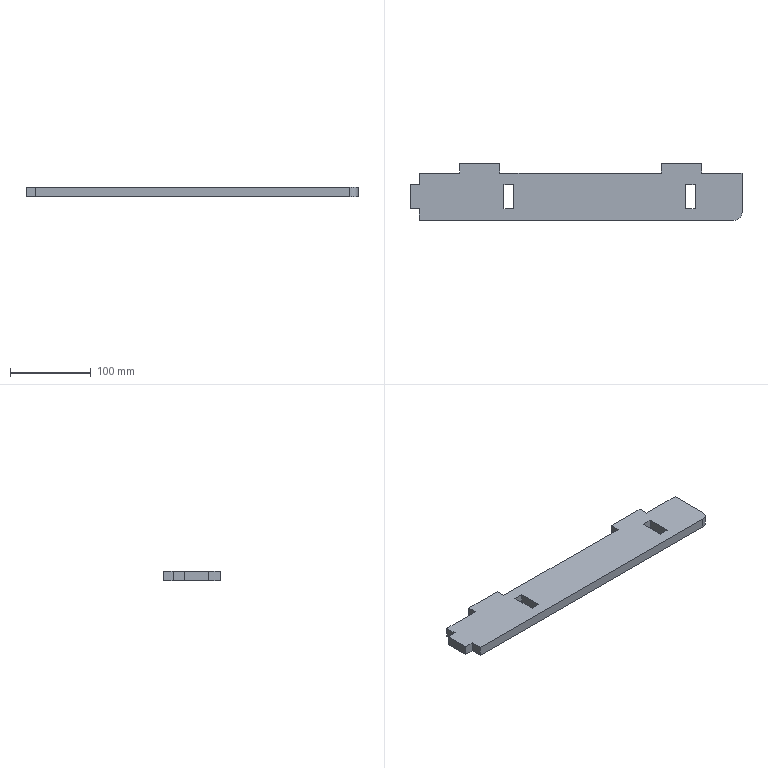Part | SolidWorks | features FlatPattern 1, SMBaseFlange 1, SheetMetal 1 | 1 solid | 27 faces | box 411.5 x 70 x 12 mm | volume 289842 mm3 | plane 26 | cylinder 1 | commonest cylinder face diameters 20 x1
STEP:
#1=CARTESIAN_POINT('',(166.972,-124.118,0.));
#2=VERTEX_POINT('',#1);
#3=CARTESIAN_POINT('',(166.972,-138.368,0.));
#4=VERTEX_POINT('',#3);
#5=CARTESIAN_POINT('',(166.972,-124.118,0.));
#6=DIRECTION('',(0.,-1.,0.));
#7=VECTOR('',#6,1000.);
#8=LINE('',#5,#7);
#9=EDGE_CURVE('',#2,#4,#8,.T.);
#10=ORIENTED_EDGE('',*,*,#9,.F.);
#11=CARTESIAN_POINT('',(166.972,-124.118,-12.));
#12=VERTEX_POINT('',#11);
#13=CARTESIAN_POINT('',(166.972,-124.118,-12.));
#14=DIRECTION('',(0.,0.,1.));
#15=VECTOR('',#14,1000.);
#16=LINE('',#13,#15);
#17=EDGE_CURVE('',#12,#2,#16,.T.);
#18=ORIENTED_EDGE('',*,*,#17,.F.);
#19=CARTESIAN_POINT('',(166.972,-138.368,-12.));
#20=VERTEX_POINT('',#19);
#21=CARTESIAN_POINT('',(166.972,-124.118,-12.));
#22=DIRECTION('',(0.,-1.,0.));
#23=VECTOR('',#22,1000.);
#24=LINE('',#21,#23);
#25=EDGE_CURVE('',#12,#20,#24,.T.);
#26=ORIENTED_EDGE('',*,*,#25,.T.);
#27=CARTESIAN_POINT('',(166.972,-138.368,-12.));
#28=DIRECTION('',(0.,0.,1.));
#29=VECTOR('',#28,1000.);
#30=LINE('',#27,#29);
#31=EDGE_CURVE('',#20,#4,#30,.T.);
#32=ORIENTED_EDGE('',*,*,#31,.T.);
#33=EDGE_LOOP('',(#10,#18,#26,#32));
#34=FACE_OUTER_BOUND('',#33,.T.);
#35=CARTESIAN_POINT('',(166.972,-124.118,-12.));
#36=DIRECTION('',(-1.,0.,0.));
#37=DIRECTION('',(0.,0.,1.));
#38=AXIS2_PLACEMENT_3D('',#35,#36,#37);
#39=PLANE('',#38);
#40=ADVANCED_FACE('',(#34),#39,.T.);
#41=CARTESIAN_POINT('',(216.972,-124.118,0.));
#42=VERTEX_POINT('',#41);
#43=CARTESIAN_POINT('',(166.972,-124.118,0.));
#44=DIRECTION('',(-1.,0.,0.));
#45=VECTOR('',#44,1000.);
#46=LINE('',#43,#45);
#47=EDGE_CURVE('',#42,#2,#46,.T.);
#48=ORIENTED_EDGE('',*,*,#47,.F.);
#49=CARTESIAN_POINT('',(216.972,-124.118,-12.));
#50=VERTEX_POINT('',#49);
#51=CARTESIAN_POINT('',(216.972,-124.118,-12.));
#52=DIRECTION('',(0.,0.,1.));
#53=VECTOR('',#52,1000.);
#54=LINE('',#51,#53);
#55=EDGE_CURVE('',#50,#42,#54,.T.);
#56=ORIENTED_EDGE('',*,*,#55,.F.);
#57=CARTESIAN_POINT('',(166.972,-124.118,-12.));
#58=DIRECTION('',(-1.,0.,0.));
#59=VECTOR('',#58,1000.);
#60=LINE('',#57,#59);
#61=EDGE_CURVE('',#50,#12,#60,.T.);
#62=ORIENTED_EDGE('',*,*,#61,.T.);
#63=ORIENTED_EDGE('',*,*,#17,.T.);
#64=EDGE_LOOP('',(#48,#56,#62,#63));
#65=FACE_OUTER_BOUND('',#64,.T.);
#66=CARTESIAN_POINT('',(166.972,-124.118,-12.));
#67=DIRECTION('',(0.,1.,0.));
#68=DIRECTION('',(-1.,0.,0.));
#69=AXIS2_PLACEMENT_3D('',#66,#67,#68);
#70=PLANE('',#69);
#71=ADVANCED_FACE('',(#65),#70,.T.);
#72=CARTESIAN_POINT('',(216.972,-112.618,0.));
#73=VERTEX_POINT('',#72);
#74=CARTESIAN_POINT('',(216.972,-112.618,0.));
#75=DIRECTION('',(0.,-1.,0.));
#76=VECTOR('',#75,1000.);
#77=LINE('',#74,#76);
#78=EDGE_CURVE('',#73,#42,#77,.T.);
#79=ORIENTED_EDGE('',*,*,#78,.F.);
#80=CARTESIAN_POINT('',(216.972,-112.618,-12.));
#81=VERTEX_POINT('',#80);
#82=CARTESIAN_POINT('',(216.972,-112.618,-12.));
#83=DIRECTION('',(0.,0.,1.));
#84=VECTOR('',#83,1000.);
#85=LINE('',#82,#84);
#86=EDGE_CURVE('',#81,#73,#85,.T.);
#87=ORIENTED_EDGE('',*,*,#86,.F.);
#88=CARTESIAN_POINT('',(216.972,-112.618,-12.));
#89=DIRECTION('',(0.,-1.,0.));
#90=VECTOR('',#89,1000.);
#91=LINE('',#88,#90);
#92=EDGE_CURVE('',#81,#50,#91,.T.);
#93=ORIENTED_EDGE('',*,*,#92,.T.);
#94=ORIENTED_EDGE('',*,*,#55,.T.);
#95=EDGE_LOOP('',(#79,#87,#93,#94));
#96=FACE_OUTER_BOUND('',#95,.T.);
#97=CARTESIAN_POINT('',(216.972,-112.618,-12.));
#98=DIRECTION('',(-1.,0.,0.));
#99=DIRECTION('',(0.,0.,1.));
#100=AXIS2_PLACEMENT_3D('',#97,#98,#99);
#101=PLANE('',#100);
#102=ADVANCED_FACE('',(#96),#101,.T.);
#103=CARTESIAN_POINT('',(266.972,-112.618,0.));
#104=VERTEX_POINT('',#103);
#105=CARTESIAN_POINT('',(266.972,-112.618,0.));
#106=DIRECTION('',(-1.,0.,0.));
#107=VECTOR('',#106,1000.);
#108=LINE('',#105,#107);
#109=EDGE_CURVE('',#104,#73,#108,.T.);
#110=ORIENTED_EDGE('',*,*,#109,.F.);
#111=CARTESIAN_POINT('',(266.972,-112.618,-12.));
#112=VERTEX_POINT('',#111);
#113=CARTESIAN_POINT('',(266.972,-112.618,-12.));
#114=DIRECTION('',(0.,0.,1.));
#115=VECTOR('',#114,1000.);
#116=LINE('',#113,#115);
#117=EDGE_CURVE('',#112,#104,#116,.T.);
#118=ORIENTED_EDGE('',*,*,#117,.F.);
#119=CARTESIAN_POINT('',(266.972,-112.618,-12.));
#120=DIRECTION('',(-1.,0.,0.));
#121=VECTOR('',#120,1000.);
#122=LINE('',#119,#121);
#123=EDGE_CURVE('',#112,#81,#122,.T.);
#124=ORIENTED_EDGE('',*,*,#123,.T.);
#125=ORIENTED_EDGE('',*,*,#86,.T.);
#126=EDGE_LOOP('',(#110,#118,#124,#125));
#127=FACE_OUTER_BOUND('',#126,.T.);
#128=CARTESIAN_POINT('',(266.972,-112.618,-12.));
#129=DIRECTION('',(0.,1.,0.));
#130=DIRECTION('',(0.,0.,1.));
#131=AXIS2_PLACEMENT_3D('',#128,#129,#130);
#132=PLANE('',#131);
#133=ADVANCED_FACE('',(#127),#132,.T.);
#134=CARTESIAN_POINT('',(266.972,-124.118,0.));
#135=VERTEX_POINT('',#134);
#136=CARTESIAN_POINT('',(266.972,-124.118,0.));
#137=DIRECTION('',(0.,1.,0.));
#138=VECTOR('',#137,1000.);
#139=LINE('',#136,#138);
#140=EDGE_CURVE('',#135,#104,#139,.T.);
#141=ORIENTED_EDGE('',*,*,#140,.F.);
#142=CARTESIAN_POINT('',(266.972,-124.118,-12.));
#143=VERTEX_POINT('',#142);
#144=CARTESIAN_POINT('',(266.972,-124.118,-12.));
#145=DIRECTION('',(0.,0.,1.));
#146=VECTOR('',#145,1000.);
#147=LINE('',#144,#146);
#148=EDGE_CURVE('',#143,#135,#147,.T.);
#149=ORIENTED_EDGE('',*,*,#148,.F.);
#150=CARTESIAN_POINT('',(266.972,-124.118,-12.));
#151=DIRECTION('',(0.,1.,0.));
#152=VECTOR('',#151,1000.);
#153=LINE('',#150,#152);
#154=EDGE_CURVE('',#143,#112,#153,.T.);
#155=ORIENTED_EDGE('',*,*,#154,.T.);
#156=ORIENTED_EDGE('',*,*,#117,.T.);
#157=EDGE_LOOP('',(#141,#149,#155,#156));
#158=FACE_OUTER_BOUND('',#157,.T.);
#159=CARTESIAN_POINT('',(266.972,-124.118,-12.));
#160=DIRECTION('',(1.,0.,0.));
#161=DIRECTION('',(0.,1.,0.));
#162=AXIS2_PLACEMENT_3D('',#159,#160,#161);
#163=PLANE('',#162);
#164=ADVANCED_FACE('',(#158),#163,.T.);
#165=CARTESIAN_POINT('',(466.972,-124.118,0.));
#166=VERTEX_POINT('',#165);
#167=CARTESIAN_POINT('',(266.972,-124.118,0.));
#168=DIRECTION('',(-1.,0.,0.));
#169=VECTOR('',#168,1000.);
#170=LINE('',#167,#169);
#171=EDGE_CURVE('',#166,#135,#170,.T.);
#172=ORIENTED_EDGE('',*,*,#171,.F.);
#173=CARTESIAN_POINT('',(466.972,-124.118,-12.));
#174=VERTEX_POINT('',#173);
#175=CARTESIAN_POINT('',(466.972,-124.118,-12.));
#176=DIRECTION('',(0.,0.,1.));
#177=VECTOR('',#176,1000.);
#178=LINE('',#175,#177);
#179=EDGE_CURVE('',#174,#166,#178,.T.);
#180=ORIENTED_EDGE('',*,*,#179,.F.);
#181=CARTESIAN_POINT('',(266.972,-124.118,-12.));
#182=DIRECTION('',(-1.,0.,0.));
#183=VECTOR('',#182,1000.);
#184=LINE('',#181,#183);
#185=EDGE_CURVE('',#174,#143,#184,.T.);
#186=ORIENTED_EDGE('',*,*,#185,.T.);
#187=ORIENTED_EDGE('',*,*,#148,.T.);
#188=EDGE_LOOP('',(#172,#180,#186,#187));
#189=FACE_OUTER_BOUND('',#188,.T.);
#190=CARTESIAN_POINT('',(266.972,-124.118,-12.));
#191=DIRECTION('',(0.,1.,0.));
#192=DIRECTION('',(0.,0.,1.));
#193=AXIS2_PLACEMENT_3D('',#190,#191,#192);
#194=PLANE('',#193);
#195=ADVANCED_FACE('',(#189),#194,.T.);
#196=CARTESIAN_POINT('',(466.972,-112.618,0.));
#197=VERTEX_POINT('',#196);
#198=CARTESIAN_POINT('',(466.972,-112.618,0.));
#199=DIRECTION('',(0.,-1.,0.));
#200=VECTOR('',#199,1000.);
#201=LINE('',#198,#200);
#202=EDGE_CURVE('',#197,#166,#201,.T.);
#203=ORIENTED_EDGE('',*,*,#202,.F.);
#204=CARTESIAN_POINT('',(466.972,-112.618,-12.));
#205=VERTEX_POINT('',#204);
#206=CARTESIAN_POINT('',(466.972,-112.618,-12.));
#207=DIRECTION('',(0.,0.,1.));
#208=VECTOR('',#207,1000.);
#209=LINE('',#206,#208);
#210=EDGE_CURVE('',#205,#197,#209,.T.);
#211=ORIENTED_EDGE('',*,*,#210,.F.);
#212=CARTESIAN_POINT('',(466.972,-112.618,-12.));
#213=DIRECTION('',(0.,-1.,0.));
#214=VECTOR('',#213,1000.);
#215=LINE('',#212,#214);
#216=EDGE_CURVE('',#205,#174,#215,.T.);
#217=ORIENTED_EDGE('',*,*,#216,.T.);
#218=ORIENTED_EDGE('',*,*,#179,.T.);
#219=EDGE_LOOP('',(#203,#211,#217,#218));
#220=FACE_OUTER_BOUND('',#219,.T.);
#221=CARTESIAN_POINT('',(466.972,-112.618,-12.));
#222=DIRECTION('',(-1.,0.,0.));
#223=DIRECTION('',(0.,0.,1.));
#224=AXIS2_PLACEMENT_3D('',#221,#222,#223);
#225=PLANE('',#224);
#226=ADVANCED_FACE('',(#220),#225,.T.);
#227=CARTESIAN_POINT('',(516.972,-112.618,0.));
#228=VERTEX_POINT('',#227);
#229=CARTESIAN_POINT('',(516.972,-112.618,0.));
#230=DIRECTION('',(-1.,0.,0.));
#231=VECTOR('',#230,1000.);
#232=LINE('',#229,#231);
#233=EDGE_CURVE('',#228,#197,#232,.T.);
#234=ORIENTED_EDGE('',*,*,#233,.F.);
#235=CARTESIAN_POINT('',(516.972,-112.618,-12.));
#236=VERTEX_POINT('',#235);
#237=CARTESIAN_POINT('',(516.972,-112.618,-12.));
#238=DIRECTION('',(0.,0.,1.));
#239=VECTOR('',#238,1000.);
#240=LINE('',#237,#239);
#241=EDGE_CURVE('',#236,#228,#240,.T.);
#242=ORIENTED_EDGE('',*,*,#241,.F.);
#243=CARTESIAN_POINT('',(516.972,-112.618,-12.));
#244=DIRECTION('',(-1.,0.,0.));
#245=VECTOR('',#244,1000.);
#246=LINE('',#243,#245);
#247=EDGE_CURVE('',#236,#205,#246,.T.);
#248=ORIENTED_EDGE('',*,*,#247,.T.);
#249=ORIENTED_EDGE('',*,*,#210,.T.);
#250=EDGE_LOOP('',(#234,#242,#248,#249));
#251=FACE_OUTER_BOUND('',#250,.T.);
#252=CARTESIAN_POINT('',(516.972,-112.618,-12.));
#253=DIRECTION('',(0.,1.,0.));
#254=DIRECTION('',(-1.,0.,0.));
#255=AXIS2_PLACEMENT_3D('',#252,#253,#254);
#256=PLANE('',#255);
#257=ADVANCED_FACE('',(#251),#256,.T.);
#258=CARTESIAN_POINT('',(516.972,-124.118,0.));
#259=VERTEX_POINT('',#258);
#260=CARTESIAN_POINT('',(516.972,-124.118,0.));
#261=DIRECTION('',(0.,1.,0.));
#262=VECTOR('',#261,1000.);
#263=LINE('',#260,#262);
#264=EDGE_CURVE('',#259,#228,#263,.T.);
#265=ORIENTED_EDGE('',*,*,#264,.F.);
#266=CARTESIAN_POINT('',(516.972,-124.118,-12.));
#267=VERTEX_POINT('',#266);
#268=CARTESIAN_POINT('',(516.972,-124.118,-12.));
#269=DIRECTION('',(0.,0.,1.));
#270=VECTOR('',#269,1000.);
#271=LINE('',#268,#270);
#272=EDGE_CURVE('',#267,#259,#271,.T.);
#273=ORIENTED_EDGE('',*,*,#272,.F.);
#274=CARTESIAN_POINT('',(516.972,-124.118,-12.));
#275=DIRECTION('',(0.,1.,0.));
#276=VECTOR('',#275,1000.);
#277=LINE('',#274,#276);
#278=EDGE_CURVE('',#267,#236,#277,.T.);
#279=ORIENTED_EDGE('',*,*,#278,.T.);
#280=ORIENTED_EDGE('',*,*,#241,.T.);
#281=EDGE_LOOP('',(#265,#273,#279,#280));
#282=FACE_OUTER_BOUND('',#281,.T.);
#283=CARTESIAN_POINT('',(516.972,-124.118,-12.));
#284=DIRECTION('',(1.,0.,0.));
#285=DIRECTION('',(0.,0.,-1.));
#286=AXIS2_PLACEMENT_3D('',#283,#284,#285);
#287=PLANE('',#286);
#288=ADVANCED_FACE('',(#282),#287,.T.);
#289=CARTESIAN_POINT('',(566.972,-124.118,0.));
#290=VERTEX_POINT('',#289);
#291=CARTESIAN_POINT('',(516.972,-124.118,0.));
#292=DIRECTION('',(-1.,0.,0.));
#293=VECTOR('',#292,1000.);
#294=LINE('',#291,#293);
#295=EDGE_CURVE('',#290,#259,#294,.T.);
#296=ORIENTED_EDGE('',*,*,#295,.F.);
#297=CARTESIAN_POINT('',(566.972,-124.118,-12.));
#298=VERTEX_POINT('',#297);
#299=CARTESIAN_POINT('',(566.972,-124.118,-12.));
#300=DIRECTION('',(0.,0.,1.));
#301=VECTOR('',#300,1000.);
#302=LINE('',#299,#301);
#303=EDGE_CURVE('',#298,#290,#302,.T.);
#304=ORIENTED_EDGE('',*,*,#303,.F.);
#305=CARTESIAN_POINT('',(516.972,-124.118,-12.));
#306=DIRECTION('',(-1.,0.,0.));
#307=VECTOR('',#306,1000.);
#308=LINE('',#305,#307);
#309=EDGE_CURVE('',#298,#267,#308,.T.);
#310=ORIENTED_EDGE('',*,*,#309,.T.);
#311=ORIENTED_EDGE('',*,*,#272,.T.);
#312=EDGE_LOOP('',(#296,#304,#310,#311));
#313=FACE_OUTER_BOUND('',#312,.T.);
#314=CARTESIAN_POINT('',(516.972,-124.118,-12.));
#315=DIRECTION('',(0.,1.,0.));
#316=DIRECTION('',(0.,0.,1.));
#317=AXIS2_PLACEMENT_3D('',#314,#315,#316);
#318=PLANE('',#317);
#319=ADVANCED_FACE('',(#313),#318,.T.);
#320=CARTESIAN_POINT('',(566.972,-172.618,0.));
#321=VERTEX_POINT('',#320);
#322=CARTESIAN_POINT('',(566.972,-124.118,0.));
#323=DIRECTION('',(0.,1.,0.));
#324=VECTOR('',#323,1000.);
#325=LINE('',#322,#324);
#326=EDGE_CURVE('',#321,#290,#325,.T.);
#327=ORIENTED_EDGE('',*,*,#326,.F.);
#328=CARTESIAN_POINT('',(566.972,-172.618,-12.));
#329=VERTEX_POINT('',#328);
#330=CARTESIAN_POINT('',(566.972,-172.618,-12.));
#331=DIRECTION('',(0.,0.,1.));
#332=VECTOR('',#331,1000.);
#333=LINE('',#330,#332);
#334=EDGE_CURVE('',#329,#321,#333,.T.);
#335=ORIENTED_EDGE('',*,*,#334,.F.);
#336=CARTESIAN_POINT('',(566.972,-124.118,-12.));
#337=DIRECTION('',(0.,1.,0.));
#338=VECTOR('',#337,1000.);
#339=LINE('',#336,#338);
#340=EDGE_CURVE('',#329,#298,#339,.T.);
#341=ORIENTED_EDGE('',*,*,#340,.T.);
#342=ORIENTED_EDGE('',*,*,#303,.T.);
#343=EDGE_LOOP('',(#327,#335,#341,#342));
#344=FACE_OUTER_BOUND('',#343,.T.);
#345=CARTESIAN_POINT('',(566.972,-124.118,-12.));
#346=DIRECTION('',(1.,0.,0.));
#347=DIRECTION('',(0.,0.,-1.));
#348=AXIS2_PLACEMENT_3D('',#345,#346,#347);
#349=PLANE('',#348);
#350=ADVANCED_FACE('',(#344),#349,.T.);
#351=CARTESIAN_POINT('',(556.972,-182.618,0.));
#352=VERTEX_POINT('',#351);
#353=CARTESIAN_POINT('',(556.972,-172.618,0.));
#354=DIRECTION('',(0.,0.,1.));
#355=DIRECTION('',(1.,0.,0.));
#356=AXIS2_PLACEMENT_3D('',#353,#354,#355);
#357=CIRCLE('',#356,10.);
#358=EDGE_CURVE('',#352,#321,#357,.T.);
#359=ORIENTED_EDGE('',*,*,#358,.F.);
#360=CARTESIAN_POINT('',(556.972,-182.618,-12.));
#361=VERTEX_POINT('',#360);
#362=CARTESIAN_POINT('',(556.972,-182.618,-12.));
#363=DIRECTION('',(0.,0.,1.));
#364=VECTOR('',#363,1000.);
#365=LINE('',#362,#364);
#366=EDGE_CURVE('',#361,#352,#365,.T.);
#367=ORIENTED_EDGE('',*,*,#366,.F.);
#368=CARTESIAN_POINT('',(556.972,-172.618,-12.));
#369=DIRECTION('',(0.,0.,1.));
#370=DIRECTION('',(1.,0.,0.));
#371=AXIS2_PLACEMENT_3D('',#368,#369,#370);
#372=CIRCLE('',#371,10.);
#373=EDGE_CURVE('',#361,#329,#372,.T.);
#374=ORIENTED_EDGE('',*,*,#373,.T.);
#375=ORIENTED_EDGE('',*,*,#334,.T.);
#376=EDGE_LOOP('',(#359,#367,#374,#375));
#377=FACE_OUTER_BOUND('',#376,.T.);
#378=CARTESIAN_POINT('',(556.972,-172.618,-12.));
#379=DIRECTION('',(0.,0.,1.));
#380=DIRECTION('',(1.,0.,0.));
#381=AXIS2_PLACEMENT_3D('',#378,#379,#380);
#382=CYLINDRICAL_SURFACE('',#381,10.);
#383=ADVANCED_FACE('',(#377),#382,.T.);
#384=CARTESIAN_POINT('',(166.972,-182.618,0.));
#385=VERTEX_POINT('',#384);
#386=CARTESIAN_POINT('',(166.972,-182.618,0.));
#387=DIRECTION('',(1.,0.,0.));
#388=VECTOR('',#387,1000.);
#389=LINE('',#386,#388);
#390=EDGE_CURVE('',#385,#352,#389,.T.);
#391=ORIENTED_EDGE('',*,*,#390,.F.);
#392=CARTESIAN_POINT('',(166.972,-182.618,-12.));
#393=VERTEX_POINT('',#392);
#394=CARTESIAN_POINT('',(166.972,-182.618,-12.));
#395=DIRECTION('',(0.,0.,1.));
#396=VECTOR('',#395,1000.);
#397=LINE('',#394,#396);
#398=EDGE_CURVE('',#393,#385,#397,.T.);
#399=ORIENTED_EDGE('',*,*,#398,.F.);
#400=CARTESIAN_POINT('',(166.972,-182.618,-12.));
#401=DIRECTION('',(1.,0.,0.));
#402=VECTOR('',#401,1000.);
#403=LINE('',#400,#402);
#404=EDGE_CURVE('',#393,#361,#403,.T.);
#405=ORIENTED_EDGE('',*,*,#404,.T.);
#406=ORIENTED_EDGE('',*,*,#366,.T.);
#407=EDGE_LOOP('',(#391,#399,#405,#406));
#408=FACE_OUTER_BOUND('',#407,.T.);
#409=CARTESIAN_POINT('',(166.972,-182.618,-12.));
#410=DIRECTION('',(0.,-1.,0.));
#411=DIRECTION('',(0.,0.,-1.));
#412=AXIS2_PLACEMENT_3D('',#409,#410,#411);
#413=PLANE('',#412);
#414=ADVANCED_FACE('',(#408),#413,.T.);
#415=CARTESIAN_POINT('',(166.972,-168.368,0.));
#416=VERTEX_POINT('',#415);
#417=CARTESIAN_POINT('',(166.972,-168.368,0.));
#418=DIRECTION('',(0.,-1.,0.));
#419=VECTOR('',#418,1000.);
#420=LINE('',#417,#419);
#421=EDGE_CURVE('',#416,#385,#420,.T.);
#422=ORIENTED_EDGE('',*,*,#421,.F.);
#423=CARTESIAN_POINT('',(166.972,-168.368,-12.));
#424=VERTEX_POINT('',#423);
#425=CARTESIAN_POINT('',(166.972,-168.368,-12.));
#426=DIRECTION('',(0.,0.,1.));
#427=VECTOR('',#426,1000.);
#428=LINE('',#425,#427);
#429=EDGE_CURVE('',#424,#416,#428,.T.);
#430=ORIENTED_EDGE('',*,*,#429,.F.);
#431=CARTESIAN_POINT('',(166.972,-168.368,-12.));
#432=DIRECTION('',(0.,-1.,0.));
#433=VECTOR('',#432,1000.);
#434=LINE('',#431,#433);
#435=EDGE_CURVE('',#424,#393,#434,.T.);
#436=ORIENTED_EDGE('',*,*,#435,.T.);
#437=ORIENTED_EDGE('',*,*,#398,.T.);
#438=EDGE_LOOP('',(#422,#430,#436,#437));
#439=FACE_OUTER_BOUND('',#438,.T.);
#440=CARTESIAN_POINT('',(166.972,-168.368,-12.));
#441=DIRECTION('',(-1.,0.,0.));
#442=DIRECTION('',(0.,0.,1.));
#443=AXIS2_PLACEMENT_3D('',#440,#441,#442);
#444=PLANE('',#443);
#445=ADVANCED_FACE('',(#439),#444,.T.);
#446=CARTESIAN_POINT('',(155.472,-168.368,0.));
#447=VERTEX_POINT('',#446);
#448=CARTESIAN_POINT('',(155.472,-168.368,0.));
#449=DIRECTION('',(1.,0.,0.));
#450=VECTOR('',#449,1000.);
#451=LINE('',#448,#450);
#452=EDGE_CURVE('',#447,#416,#451,.T.);
#453=ORIENTED_EDGE('',*,*,#452,.F.);
#454=CARTESIAN_POINT('',(155.472,-168.368,-12.));
#455=VERTEX_POINT('',#454);
#456=CARTESIAN_POINT('',(155.472,-168.368,-12.));
#457=DIRECTION('',(0.,0.,1.));
#458=VECTOR('',#457,1000.);
#459=LINE('',#456,#458);
#460=EDGE_CURVE('',#455,#447,#459,.T.);
#461=ORIENTED_EDGE('',*,*,#460,.F.);
#462=CARTESIAN_POINT('',(155.472,-168.368,-12.));
#463=DIRECTION('',(1.,0.,0.));
#464=VECTOR('',#463,1000.);
#465=LINE('',#462,#464);
#466=EDGE_CURVE('',#455,#424,#465,.T.);
#467=ORIENTED_EDGE('',*,*,#466,.T.);
#468=ORIENTED_EDGE('',*,*,#429,.T.);
#469=EDGE_LOOP('',(#453,#461,#467,#468));
#470=FACE_OUTER_BOUND('',#469,.T.);
#471=CARTESIAN_POINT('',(155.472,-168.368,-12.));
#472=DIRECTION('',(0.,-1.,0.));
#473=DIRECTION('',(1.,0.,0.));
#474=AXIS2_PLACEMENT_3D('',#471,#472,#473);
#475=PLANE('',#474);
#476=ADVANCED_FACE('',(#470),#475,.T.);
#477=CARTESIAN_POINT('',(155.472,-138.368,0.));
#478=VERTEX_POINT('',#477);
#479=CARTESIAN_POINT('',(155.472,-138.368,0.));
#480=DIRECTION('',(0.,-1.,0.));
#481=VECTOR('',#480,1000.);
#482=LINE('',#479,#481);
#483=EDGE_CURVE('',#478,#447,#482,.T.);
#484=ORIENTED_EDGE('',*,*,#483,.F.);
#485=CARTESIAN_POINT('',(155.472,-138.368,-12.));
#486=VERTEX_POINT('',#485);
#487=CARTESIAN_POINT('',(155.472,-138.368,-12.));
#488=DIRECTION('',(0.,0.,1.));
#489=VECTOR('',#488,1000.);
#490=LINE('',#487,#489);
#491=EDGE_CURVE('',#486,#478,#490,.T.);
#492=ORIENTED_EDGE('',*,*,#491,.F.);
#493=CARTESIAN_POINT('',(155.472,-138.368,-12.));
#494=DIRECTION('',(0.,-1.,0.));
#495=VECTOR('',#494,1000.);
#496=LINE('',#493,#495);
#497=EDGE_CURVE('',#486,#455,#496,.T.);
#498=ORIENTED_EDGE('',*,*,#497,.T.);
#499=ORIENTED_EDGE('',*,*,#460,.T.);
#500=EDGE_LOOP('',(#484,#492,#498,#499));
#501=FACE_OUTER_BOUND('',#500,.T.);
#502=CARTESIAN_POINT('',(155.472,-138.368,-12.));
#503=DIRECTION('',(-1.,0.,0.));
#504=DIRECTION('',(0.,0.,1.));
#505=AXIS2_PLACEMENT_3D('',#502,#503,#504);
#506=PLANE('',#505);
#507=ADVANCED_FACE('',(#501),#506,.T.);
#508=CARTESIAN_POINT('',(166.972,-138.368,0.));
#509=DIRECTION('',(-1.,0.,0.));
#510=VECTOR('',#509,1000.);
#511=LINE('',#508,#510);
#512=EDGE_CURVE('',#4,#478,#511,.T.);
#513=ORIENTED_EDGE('',*,*,#512,.F.);
#514=ORIENTED_EDGE('',*,*,#31,.F.);
#515=CARTESIAN_POINT('',(166.972,-138.368,-12.));
#516=DIRECTION('',(-1.,0.,0.));
#517=VECTOR('',#516,1000.);
#518=LINE('',#515,#517);
#519=EDGE_CURVE('',#20,#486,#518,.T.);
#520=ORIENTED_EDGE('',*,*,#519,.T.);
#521=ORIENTED_EDGE('',*,*,#491,.T.);
#522=EDGE_LOOP('',(#513,#514,#520,#521));
#523=FACE_OUTER_BOUND('',#522,.T.);
#524=CARTESIAN_POINT('',(166.972,-138.368,-12.));
#525=DIRECTION('',(0.,1.,0.));
#526=DIRECTION('',(0.,0.,1.));
#527=AXIS2_PLACEMENT_3D('',#524,#525,#526);
#528=PLANE('',#527);
#529=ADVANCED_FACE('',(#523),#528,.T.);
#530=CARTESIAN_POINT('',(271.972,-168.368,-12.));
#531=VERTEX_POINT('',#530);
#532=CARTESIAN_POINT('',(283.972,-168.368,-12.));
#533=VERTEX_POINT('',#532);
#534=CARTESIAN_POINT('',(283.972,-168.368,-12.));
#535=DIRECTION('',(1.,0.,0.));
#536=VECTOR('',#535,1000.);
#537=LINE('',#534,#536);
#538=EDGE_CURVE('',#531,#533,#537,.T.);
#539=ORIENTED_EDGE('',*,*,#538,.T.);
#540=CARTESIAN_POINT('',(283.972,-138.368,-12.));
#541=VERTEX_POINT('',#540);
#542=CARTESIAN_POINT('',(283.972,-138.368,-12.));
#543=DIRECTION('',(0.,1.,0.));
#544=VECTOR('',#543,1000.);
#545=LINE('',#542,#544);
#546=EDGE_CURVE('',#533,#541,#545,.T.);
#547=ORIENTED_EDGE('',*,*,#546,.T.);
#548=CARTESIAN_POINT('',(271.972,-138.368,-12.));
#549=VERTEX_POINT('',#548);
#550=CARTESIAN_POINT('',(283.972,-138.368,-12.));
#551=DIRECTION('',(-1.,0.,0.));
#552=VECTOR('',#551,1000.);
#553=LINE('',#550,#552);
#554=EDGE_CURVE('',#541,#549,#553,.T.);
#555=ORIENTED_EDGE('',*,*,#554,.T.);
#556=CARTESIAN_POINT('',(271.972,-138.368,-12.));
#557=DIRECTION('',(0.,-1.,0.));
#558=VECTOR('',#557,1000.);
#559=LINE('',#556,#558);
#560=EDGE_CURVE('',#549,#531,#559,.T.);
#561=ORIENTED_EDGE('',*,*,#560,.T.);
#562=EDGE_LOOP('',(#539,#547,#555,#561));
#563=FACE_BOUND('',#562,.T.);
#564=CARTESIAN_POINT('',(508.972,-138.368,-12.));
#565=VERTEX_POINT('',#564);
#566=CARTESIAN_POINT('',(496.972,-138.368,-12.));
#567=VERTEX_POINT('',#566);
#568=CARTESIAN_POINT('',(496.972,-138.368,-12.));
#569=DIRECTION('',(-1.,0.,0.));
#570=VECTOR('',#569,1000.);
#571=LINE('',#568,#570);
#572=EDGE_CURVE('',#565,#567,#571,.T.);
#573=ORIENTED_EDGE('',*,*,#572,.T.);
#574=CARTESIAN_POINT('',(496.972,-168.368,-12.));
#575=VERTEX_POINT('',#574);
#576=CARTESIAN_POINT('',(496.972,-168.368,-12.));
#577=DIRECTION('',(0.,-1.,0.));
#578=VECTOR('',#577,1000.);
#579=LINE('',#576,#578);
#580=EDGE_CURVE('',#567,#575,#579,.T.);
#581=ORIENTED_EDGE('',*,*,#580,.T.);
#582=CARTESIAN_POINT('',(508.972,-168.368,-12.));
#583=VERTEX_POINT('',#582);
#584=CARTESIAN_POINT('',(496.972,-168.368,-12.));
#585=DIRECTION('',(1.,0.,0.));
#586=VECTOR('',#585,1000.);
#587=LINE('',#584,#586);
#588=EDGE_CURVE('',#575,#583,#587,.T.);
#589=ORIENTED_EDGE('',*,*,#588,.T.);
#590=CARTESIAN_POINT('',(508.972,-168.368,-12.));
#591=DIRECTION('',(0.,1.,0.));
#592=VECTOR('',#591,1000.);
#593=LINE('',#590,#592);
#594=EDGE_CURVE('',#583,#565,#593,.T.);
#595=ORIENTED_EDGE('',*,*,#594,.T.);
#596=EDGE_LOOP('',(#573,#581,#589,#595));
#597=FACE_BOUND('',#596,.T.);
#598=ORIENTED_EDGE('',*,*,#25,.F.);
#599=ORIENTED_EDGE('',*,*,#61,.F.);
#600=ORIENTED_EDGE('',*,*,#92,.F.);
#601=ORIENTED_EDGE('',*,*,#123,.F.);
#602=ORIENTED_EDGE('',*,*,#154,.F.);
#603=ORIENTED_EDGE('',*,*,#185,.F.);
#604=ORIENTED_EDGE('',*,*,#216,.F.);
#605=ORIENTED_EDGE('',*,*,#247,.F.);
#606=ORIENTED_EDGE('',*,*,#278,.F.);
#607=ORIENTED_EDGE('',*,*,#309,.F.);
#608=ORIENTED_EDGE('',*,*,#340,.F.);
#609=ORIENTED_EDGE('',*,*,#373,.F.);
#610=ORIENTED_EDGE('',*,*,#404,.F.);
#611=ORIENTED_EDGE('',*,*,#435,.F.);
#612=ORIENTED_EDGE('',*,*,#466,.F.);
#613=ORIENTED_EDGE('',*,*,#497,.F.);
#614=ORIENTED_EDGE('',*,*,#519,.F.);
#615=EDGE_LOOP('',(#598,#599,#600,#601,#602,#603,#604,#605,#606,#607,#608,#609,#610,#611,#612,#613,#614));
#616=FACE_OUTER_BOUND('',#615,.T.);
#617=CARTESIAN_POINT('',(556.972,-172.618,-12.));
#618=DIRECTION('',(0.,0.,1.));
#619=DIRECTION('',(1.,0.,0.));
#620=AXIS2_PLACEMENT_3D('',#617,#618,#619);
#621=PLANE('',#620);
#622=ADVANCED_FACE('',(#563,#597,#616),#621,.F.);
#623=CARTESIAN_POINT('',(283.972,-168.368,0.));
#624=VERTEX_POINT('',#623);
#625=CARTESIAN_POINT('',(283.972,-138.368,0.));
#626=VERTEX_POINT('',#625);
#627=CARTESIAN_POINT('',(283.972,-138.368,0.));
#628=DIRECTION('',(0.,1.,0.));
#629=VECTOR('',#628,1000.);
#630=LINE('',#627,#629);
#631=EDGE_CURVE('',#624,#626,#630,.T.);
#632=ORIENTED_EDGE('',*,*,#631,.F.);
#633=CARTESIAN_POINT('',(271.972,-168.368,0.));
#634=VERTEX_POINT('',#633);
#635=CARTESIAN_POINT('',(283.972,-168.368,0.));
#636=DIRECTION('',(1.,0.,0.));
#637=VECTOR('',#636,1000.);
#638=LINE('',#635,#637);
#639=EDGE_CURVE('',#634,#624,#638,.T.);
#640=ORIENTED_EDGE('',*,*,#639,.F.);
#641=CARTESIAN_POINT('',(271.972,-138.368,0.));
#642=VERTEX_POINT('',#641);
#643=CARTESIAN_POINT('',(271.972,-138.368,0.));
#644=DIRECTION('',(0.,-1.,0.));
#645=VECTOR('',#644,1000.);
#646=LINE('',#643,#645);
#647=EDGE_CURVE('',#642,#634,#646,.T.);
#648=ORIENTED_EDGE('',*,*,#647,.F.);
#649=CARTESIAN_POINT('',(283.972,-138.368,0.));
#650=DIRECTION('',(-1.,0.,0.));
#651=VECTOR('',#650,1000.);
#652=LINE('',#649,#651);
#653=EDGE_CURVE('',#626,#642,#652,.T.);
#654=ORIENTED_EDGE('',*,*,#653,.F.);
#655=EDGE_LOOP('',(#632,#640,#648,#654));
#656=FACE_BOUND('',#655,.T.);
#657=CARTESIAN_POINT('',(496.972,-138.368,0.));
#658=VERTEX_POINT('',#657);
#659=CARTESIAN_POINT('',(496.972,-168.368,0.));
#660=VERTEX_POINT('',#659);
#661=CARTESIAN_POINT('',(496.972,-168.368,0.));
#662=DIRECTION('',(0.,-1.,0.));
#663=VECTOR('',#662,1000.);
#664=LINE('',#661,#663);
#665=EDGE_CURVE('',#658,#660,#664,.T.);
#666=ORIENTED_EDGE('',*,*,#665,.F.);
#667=CARTESIAN_POINT('',(508.972,-138.368,0.));
#668=VERTEX_POINT('',#667);
#669=CARTESIAN_POINT('',(496.972,-138.368,0.));
#670=DIRECTION('',(-1.,0.,0.));
#671=VECTOR('',#670,1000.);
#672=LINE('',#669,#671);
#673=EDGE_CURVE('',#668,#658,#672,.T.);
#674=ORIENTED_EDGE('',*,*,#673,.F.);
#675=CARTESIAN_POINT('',(508.972,-168.368,0.));
#676=VERTEX_POINT('',#675);
#677=CARTESIAN_POINT('',(508.972,-168.368,0.));
#678=DIRECTION('',(0.,1.,0.));
#679=VECTOR('',#678,1000.);
#680=LINE('',#677,#679);
#681=EDGE_CURVE('',#676,#668,#680,.T.);
#682=ORIENTED_EDGE('',*,*,#681,.F.);
#683=CARTESIAN_POINT('',(496.972,-168.368,0.));
#684=DIRECTION('',(1.,0.,0.));
#685=VECTOR('',#684,1000.);
#686=LINE('',#683,#685);
#687=EDGE_CURVE('',#660,#676,#686,.T.);
#688=ORIENTED_EDGE('',*,*,#687,.F.);
#689=EDGE_LOOP('',(#666,#674,#682,#688));
#690=FACE_BOUND('',#689,.T.);
#691=ORIENTED_EDGE('',*,*,#9,.T.);
#692=ORIENTED_EDGE('',*,*,#512,.T.);
#693=ORIENTED_EDGE('',*,*,#483,.T.);
#694=ORIENTED_EDGE('',*,*,#452,.T.);
#695=ORIENTED_EDGE('',*,*,#421,.T.);
#696=ORIENTED_EDGE('',*,*,#390,.T.);
#697=ORIENTED_EDGE('',*,*,#358,.T.);
#698=ORIENTED_EDGE('',*,*,#326,.T.);
#699=ORIENTED_EDGE('',*,*,#295,.T.);
#700=ORIENTED_EDGE('',*,*,#264,.T.);
#701=ORIENTED_EDGE('',*,*,#233,.T.);
#702=ORIENTED_EDGE('',*,*,#202,.T.);
#703=ORIENTED_EDGE('',*,*,#171,.T.);
#704=ORIENTED_EDGE('',*,*,#140,.T.);
#705=ORIENTED_EDGE('',*,*,#109,.T.);
#706=ORIENTED_EDGE('',*,*,#78,.T.);
#707=ORIENTED_EDGE('',*,*,#47,.T.);
#708=EDGE_LOOP('',(#691,#692,#693,#694,#695,#696,#697,#698,#699,#700,#701,#702,#703,#704,#705,#706,#707));
#709=FACE_OUTER_BOUND('',#708,.T.);
#710=CARTESIAN_POINT('',(556.972,-172.618,0.));
#711=DIRECTION('',(0.,0.,1.));
#712=DIRECTION('',(1.,0.,0.));
#713=AXIS2_PLACEMENT_3D('',#710,#711,#712);
#714=PLANE('',#713);
#715=ADVANCED_FACE('',(#656,#690,#709),#714,.T.);
#716=ORIENTED_EDGE('',*,*,#665,.T.);
#717=CARTESIAN_POINT('',(496.972,-168.368,-12.));
#718=DIRECTION('',(0.,0.,1.));
#719=VECTOR('',#718,1000.);
#720=LINE('',#717,#719);
#721=EDGE_CURVE('',#575,#660,#720,.T.);
#722=ORIENTED_EDGE('',*,*,#721,.F.);
#723=ORIENTED_EDGE('',*,*,#580,.F.);
#724=CARTESIAN_POINT('',(496.972,-138.368,-12.));
#725=DIRECTION('',(0.,0.,1.));
#726=VECTOR('',#725,1000.);
#727=LINE('',#724,#726);
#728=EDGE_CURVE('',#567,#658,#727,.T.);
#729=ORIENTED_EDGE('',*,*,#728,.T.);
#730=EDGE_LOOP('',(#716,#722,#723,#729));
#731=FACE_OUTER_BOUND('',#730,.T.);
#732=CARTESIAN_POINT('',(496.972,-168.368,-12.));
#733=DIRECTION('',(-1.,0.,0.));
#734=DIRECTION('',(0.,0.,1.));
#735=AXIS2_PLACEMENT_3D('',#732,#733,#734);
#736=PLANE('',#735);
#737=ADVANCED_FACE('',(#731),#736,.F.);
#738=ORIENTED_EDGE('',*,*,#673,.T.);
#739=ORIENTED_EDGE('',*,*,#728,.F.);
#740=ORIENTED_EDGE('',*,*,#572,.F.);
#741=CARTESIAN_POINT('',(508.972,-138.368,-12.));
#742=DIRECTION('',(0.,0.,1.));
#743=VECTOR('',#742,1000.);
#744=LINE('',#741,#743);
#745=EDGE_CURVE('',#565,#668,#744,.T.);
#746=ORIENTED_EDGE('',*,*,#745,.T.);
#747=EDGE_LOOP('',(#738,#739,#740,#746));
#748=FACE_OUTER_BOUND('',#747,.T.);
#749=CARTESIAN_POINT('',(496.972,-138.368,-12.));
#750=DIRECTION('',(0.,1.,0.));
#751=DIRECTION('',(0.,0.,1.));
#752=AXIS2_PLACEMENT_3D('',#749,#750,#751);
#753=PLANE('',#752);
#754=ADVANCED_FACE('',(#748),#753,.F.);
#755=ORIENTED_EDGE('',*,*,#681,.T.);
#756=ORIENTED_EDGE('',*,*,#745,.F.);
#757=ORIENTED_EDGE('',*,*,#594,.F.);
#758=CARTESIAN_POINT('',(508.972,-168.368,-12.));
#759=DIRECTION('',(0.,0.,1.));
#760=VECTOR('',#759,1000.);
#761=LINE('',#758,#760);
#762=EDGE_CURVE('',#583,#676,#761,.T.);
#763=ORIENTED_EDGE('',*,*,#762,.T.);
#764=EDGE_LOOP('',(#755,#756,#757,#763));
#765=FACE_OUTER_BOUND('',#764,.T.);
#766=CARTESIAN_POINT('',(508.972,-168.368,-12.));
#767=DIRECTION('',(1.,0.,0.));
#768=DIRECTION('',(0.,0.,-1.));
#769=AXIS2_PLACEMENT_3D('',#766,#767,#768);
#770=PLANE('',#769);
#771=ADVANCED_FACE('',(#765),#770,.F.);
#772=ORIENTED_EDGE('',*,*,#687,.T.);
#773=ORIENTED_EDGE('',*,*,#762,.F.);
#774=ORIENTED_EDGE('',*,*,#588,.F.);
#775=ORIENTED_EDGE('',*,*,#721,.T.);
#776=EDGE_LOOP('',(#772,#773,#774,#775));
#777=FACE_OUTER_BOUND('',#776,.T.);
#778=CARTESIAN_POINT('',(496.972,-168.368,-12.));
#779=DIRECTION('',(0.,-1.,0.));
#780=DIRECTION('',(0.,0.,-1.));
#781=AXIS2_PLACEMENT_3D('',#778,#779,#780);
#782=PLANE('',#781);
#783=ADVANCED_FACE('',(#777),#782,.F.);
#784=ORIENTED_EDGE('',*,*,#631,.T.);
#785=CARTESIAN_POINT('',(283.972,-138.368,-12.));
#786=DIRECTION('',(0.,0.,1.));
#787=VECTOR('',#786,1000.);
#788=LINE('',#785,#787);
#789=EDGE_CURVE('',#541,#626,#788,.T.);
#790=ORIENTED_EDGE('',*,*,#789,.F.);
#791=ORIENTED_EDGE('',*,*,#546,.F.);
#792=CARTESIAN_POINT('',(283.972,-168.368,-12.));
#793=DIRECTION('',(0.,0.,1.));
#794=VECTOR('',#793,1000.);
#795=LINE('',#792,#794);
#796=EDGE_CURVE('',#533,#624,#795,.T.);
#797=ORIENTED_EDGE('',*,*,#796,.T.);
#798=EDGE_LOOP('',(#784,#790,#791,#797));
#799=FACE_OUTER_BOUND('',#798,.T.);
#800=CARTESIAN_POINT('',(283.972,-138.368,-12.));
#801=DIRECTION('',(1.,0.,0.));
#802=DIRECTION('',(0.,0.,-1.));
#803=AXIS2_PLACEMENT_3D('',#800,#801,#802);
#804=PLANE('',#803);
#805=ADVANCED_FACE('',(#799),#804,.F.);
#806=ORIENTED_EDGE('',*,*,#639,.T.);
#807=ORIENTED_EDGE('',*,*,#796,.F.);
#808=ORIENTED_EDGE('',*,*,#538,.F.);
#809=CARTESIAN_POINT('',(271.972,-168.368,-12.));
#810=DIRECTION('',(0.,0.,1.));
#811=VECTOR('',#810,1000.);
#812=LINE('',#809,#811);
#813=EDGE_CURVE('',#531,#634,#812,.T.);
#814=ORIENTED_EDGE('',*,*,#813,.T.);
#815=EDGE_LOOP('',(#806,#807,#808,#814));
#816=FACE_OUTER_BOUND('',#815,.T.);
#817=CARTESIAN_POINT('',(283.972,-168.368,-12.));
#818=DIRECTION('',(0.,-1.,0.));
#819=DIRECTION('',(1.,0.,0.));
#820=AXIS2_PLACEMENT_3D('',#817,#818,#819);
#821=PLANE('',#820);
#822=ADVANCED_FACE('',(#816),#821,.F.);
#823=ORIENTED_EDGE('',*,*,#647,.T.);
#824=ORIENTED_EDGE('',*,*,#813,.F.);
#825=ORIENTED_EDGE('',*,*,#560,.F.);
#826=CARTESIAN_POINT('',(271.972,-138.368,-12.));
#827=DIRECTION('',(0.,0.,1.));
#828=VECTOR('',#827,1000.);
#829=LINE('',#826,#828);
#830=EDGE_CURVE('',#549,#642,#829,.T.);
#831=ORIENTED_EDGE('',*,*,#830,.T.);
#832=EDGE_LOOP('',(#823,#824,#825,#831));
#833=FACE_OUTER_BOUND('',#832,.T.);
#834=CARTESIAN_POINT('',(271.972,-138.368,-12.));
#835=DIRECTION('',(-1.,0.,0.));
#836=DIRECTION('',(0.,0.,1.));
#837=AXIS2_PLACEMENT_3D('',#834,#835,#836);
#838=PLANE('',#837);
#839=ADVANCED_FACE('',(#833),#838,.F.);
#840=ORIENTED_EDGE('',*,*,#653,.T.);
#841=ORIENTED_EDGE('',*,*,#830,.F.);
#842=ORIENTED_EDGE('',*,*,#554,.F.);
#843=ORIENTED_EDGE('',*,*,#789,.T.);
#844=EDGE_LOOP('',(#840,#841,#842,#843));
#845=FACE_OUTER_BOUND('',#844,.T.);
#846=CARTESIAN_POINT('',(283.972,-138.368,-12.));
#847=DIRECTION('',(0.,1.,0.));
#848=DIRECTION('',(0.,0.,1.));
#849=AXIS2_PLACEMENT_3D('',#846,#847,#848);
#850=PLANE('',#849);
#851=ADVANCED_FACE('',(#845),#850,.F.);
#852=CLOSED_SHELL('',(#40,#71,#102,#133,#164,#195,#226,#257,#288,#319,#350,#383,#414,#445,#476,#507,#529,#622,#715,#737,#754,#771,#783,#805,#822,#839,#851));
#853=MANIFOLD_SOLID_BREP('',#852);
#854=CARTESIAN_POINT('',(0.,0.,0.));
#855=DIRECTION('',(0.,0.,1.));
#856=DIRECTION('',(1.,0.,0.));
#857=AXIS2_PLACEMENT_3D('',#854,#855,#856);
#858=(LENGTH_UNIT()NAMED_UNIT(*)SI_UNIT(.MILLI.,.METRE.));
#859=UNCERTAINTY_MEASURE_WITH_UNIT(LENGTH_MEASURE(0.00001),#858,'','');
#860=(NAMED_UNIT(*)PLANE_ANGLE_UNIT()SI_UNIT($,.RADIAN.));
#861=(NAMED_UNIT(*)SI_UNIT($,.STERADIAN.)SOLID_ANGLE_UNIT());
#862=(GEOMETRIC_REPRESENTATION_CONTEXT(3)GLOBAL_UNCERTAINTY_ASSIGNED_CONTEXT((#859))GLOBAL_UNIT_ASSIGNED_CONTEXT((#858,#860,#861))REPRESENTATION_CONTEXT('',''));
#863=ADVANCED_BREP_SHAPE_REPRESENTATION('',(#853,#857),#862);